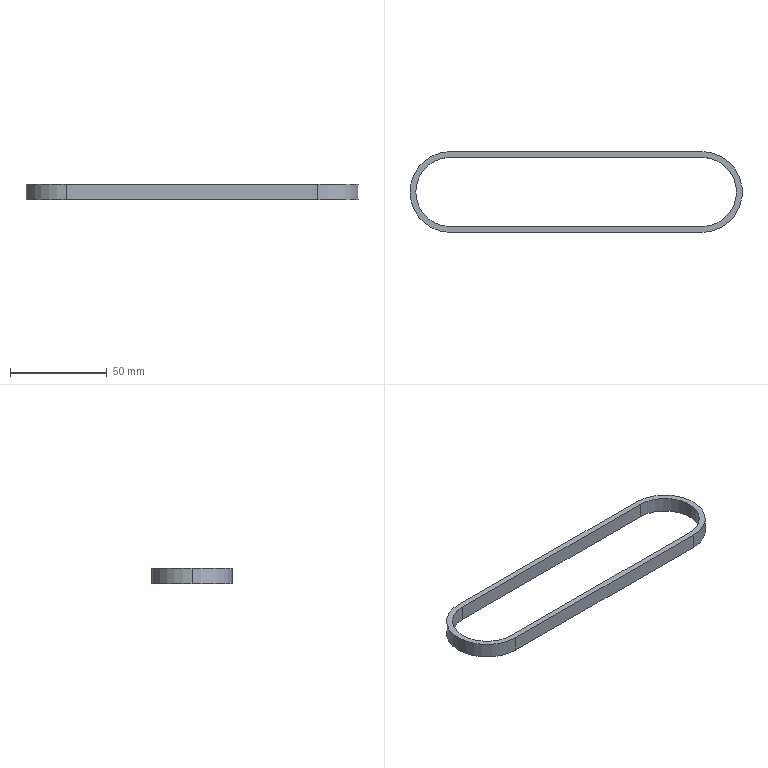Part | SolidWorks | features Extrusion 1, Shell 1 | 1 solid | 12 faces | box 171.8 x 41.8 x 7.9 mm | volume 9051 mm3 | cylinder 6 | plane 6 | commonest cylinder face diameters 35.8 x3 41.8 x3
STEP:
#1=CARTESIAN_POINT('',(-130.,17.9,7.9));
#2=VERTEX_POINT('',#1);
#3=CARTESIAN_POINT('',(-147.9,0.,7.9));
#4=VERTEX_POINT('',#3);
#5=CARTESIAN_POINT('',(-130.,0.,7.9));
#6=DIRECTION('',(0.,0.,1.));
#7=DIRECTION('',(1.,0.,0.));
#8=AXIS2_PLACEMENT_3D('',#5,#6,#7);
#9=CIRCLE('',#8,17.9);
#10=EDGE_CURVE('',#2,#4,#9,.T.);
#11=ORIENTED_EDGE('',*,*,#10,.T.);
#12=CARTESIAN_POINT('',(-147.9,0.,0.));
#13=VERTEX_POINT('',#12);
#14=CARTESIAN_POINT('',(-147.9,0.,7.9));
#15=DIRECTION('',(0.,0.,-1.));
#16=VECTOR('',#15,1000.);
#17=LINE('',#14,#16);
#18=EDGE_CURVE('',#4,#13,#17,.T.);
#19=ORIENTED_EDGE('',*,*,#18,.T.);
#20=CARTESIAN_POINT('',(-130.,17.9,0.));
#21=VERTEX_POINT('',#20);
#22=CARTESIAN_POINT('',(-130.,0.,0.));
#23=DIRECTION('',(0.,0.,1.));
#24=DIRECTION('',(1.,0.,0.));
#25=AXIS2_PLACEMENT_3D('',#22,#23,#24);
#26=CIRCLE('',#25,17.9);
#27=EDGE_CURVE('',#21,#13,#26,.T.);
#28=ORIENTED_EDGE('',*,*,#27,.F.);
#29=CARTESIAN_POINT('',(-130.,17.9,7.9));
#30=DIRECTION('',(0.,0.,-1.));
#31=VECTOR('',#30,1000.);
#32=LINE('',#29,#31);
#33=EDGE_CURVE('',#2,#21,#32,.T.);
#34=ORIENTED_EDGE('',*,*,#33,.F.);
#35=EDGE_LOOP('',(#11,#19,#28,#34));
#36=FACE_OUTER_BOUND('',#35,.T.);
#37=CARTESIAN_POINT('',(-130.,0.,7.9));
#38=DIRECTION('',(0.,0.,-1.));
#39=DIRECTION('',(-1.,0.,0.));
#40=AXIS2_PLACEMENT_3D('',#37,#38,#39);
#41=CYLINDRICAL_SURFACE('',#40,17.9);
#42=ADVANCED_FACE('',(#36),#41,.F.);
#43=CARTESIAN_POINT('',(-150.9,0.,7.9));
#44=VERTEX_POINT('',#43);
#45=CARTESIAN_POINT('',(-130.,-20.9,7.9));
#46=VERTEX_POINT('',#45);
#47=CARTESIAN_POINT('',(-130.,0.,7.9));
#48=DIRECTION('',(0.,0.,1.));
#49=DIRECTION('',(1.,0.,0.));
#50=AXIS2_PLACEMENT_3D('',#47,#48,#49);
#51=CIRCLE('',#50,20.9);
#52=EDGE_CURVE('',#44,#46,#51,.T.);
#53=ORIENTED_EDGE('',*,*,#52,.F.);
#54=CARTESIAN_POINT('',(-150.9,0.,0.));
#55=VERTEX_POINT('',#54);
#56=CARTESIAN_POINT('',(-150.9,0.,7.9));
#57=DIRECTION('',(0.,0.,-1.));
#58=VECTOR('',#57,1000.);
#59=LINE('',#56,#58);
#60=EDGE_CURVE('',#44,#55,#59,.T.);
#61=ORIENTED_EDGE('',*,*,#60,.T.);
#62=CARTESIAN_POINT('',(-130.,-20.9,0.));
#63=VERTEX_POINT('',#62);
#64=CARTESIAN_POINT('',(-130.,0.,0.));
#65=DIRECTION('',(0.,0.,1.));
#66=DIRECTION('',(1.,0.,0.));
#67=AXIS2_PLACEMENT_3D('',#64,#65,#66);
#68=CIRCLE('',#67,20.9);
#69=EDGE_CURVE('',#55,#63,#68,.T.);
#70=ORIENTED_EDGE('',*,*,#69,.T.);
#71=CARTESIAN_POINT('',(-130.,-20.9,7.9));
#72=DIRECTION('',(0.,0.,-1.));
#73=VECTOR('',#72,1000.);
#74=LINE('',#71,#73);
#75=EDGE_CURVE('',#46,#63,#74,.T.);
#76=ORIENTED_EDGE('',*,*,#75,.F.);
#77=EDGE_LOOP('',(#53,#61,#70,#76));
#78=FACE_OUTER_BOUND('',#77,.T.);
#79=CARTESIAN_POINT('',(-130.,0.,7.9));
#80=DIRECTION('',(0.,0.,-1.));
#81=DIRECTION('',(-1.,0.,0.));
#82=AXIS2_PLACEMENT_3D('',#79,#80,#81);
#83=CYLINDRICAL_SURFACE('',#82,20.9);
#84=ADVANCED_FACE('',(#78),#83,.T.);
#85=CARTESIAN_POINT('',(0.,-20.9,0.));
#86=VERTEX_POINT('',#85);
#87=CARTESIAN_POINT('',(0.,20.9,0.));
#88=VERTEX_POINT('',#87);
#89=CARTESIAN_POINT('',(0.,0.,0.));
#90=DIRECTION('',(0.,0.,1.));
#91=DIRECTION('',(1.,0.,0.));
#92=AXIS2_PLACEMENT_3D('',#89,#90,#91);
#93=CIRCLE('',#92,20.9);
#94=EDGE_CURVE('',#86,#88,#93,.T.);
#95=ORIENTED_EDGE('',*,*,#94,.T.);
#96=CARTESIAN_POINT('',(0.,20.9,7.9));
#97=VERTEX_POINT('',#96);
#98=CARTESIAN_POINT('',(0.,20.9,7.9));
#99=DIRECTION('',(0.,0.,-1.));
#100=VECTOR('',#99,1000.);
#101=LINE('',#98,#100);
#102=EDGE_CURVE('',#97,#88,#101,.T.);
#103=ORIENTED_EDGE('',*,*,#102,.F.);
#104=CARTESIAN_POINT('',(0.,-20.9,7.9));
#105=VERTEX_POINT('',#104);
#106=CARTESIAN_POINT('',(0.,0.,7.9));
#107=DIRECTION('',(0.,0.,1.));
#108=DIRECTION('',(1.,0.,0.));
#109=AXIS2_PLACEMENT_3D('',#106,#107,#108);
#110=CIRCLE('',#109,20.9);
#111=EDGE_CURVE('',#105,#97,#110,.T.);
#112=ORIENTED_EDGE('',*,*,#111,.F.);
#113=CARTESIAN_POINT('',(0.,-20.9,7.9));
#114=DIRECTION('',(0.,0.,-1.));
#115=VECTOR('',#114,1000.);
#116=LINE('',#113,#115);
#117=EDGE_CURVE('',#105,#86,#116,.T.);
#118=ORIENTED_EDGE('',*,*,#117,.T.);
#119=EDGE_LOOP('',(#95,#103,#112,#118));
#120=FACE_OUTER_BOUND('',#119,.T.);
#121=CARTESIAN_POINT('',(0.,0.,7.9));
#122=DIRECTION('',(0.,0.,-1.));
#123=DIRECTION('',(-1.,0.,0.));
#124=AXIS2_PLACEMENT_3D('',#121,#122,#123);
#125=CYLINDRICAL_SURFACE('',#124,20.9);
#126=ADVANCED_FACE('',(#120),#125,.T.);
#127=CARTESIAN_POINT('',(-130.,20.9,0.));
#128=VERTEX_POINT('',#127);
#129=CARTESIAN_POINT('',(0.,20.9,0.));
#130=DIRECTION('',(-1.,0.,0.));
#131=VECTOR('',#130,1000.);
#132=LINE('',#129,#131);
#133=EDGE_CURVE('',#88,#128,#132,.T.);
#134=ORIENTED_EDGE('',*,*,#133,.T.);
#135=CARTESIAN_POINT('',(-130.,20.9,7.9));
#136=VERTEX_POINT('',#135);
#137=CARTESIAN_POINT('',(-130.,20.9,7.9));
#138=DIRECTION('',(0.,0.,-1.));
#139=VECTOR('',#138,1000.);
#140=LINE('',#137,#139);
#141=EDGE_CURVE('',#136,#128,#140,.T.);
#142=ORIENTED_EDGE('',*,*,#141,.F.);
#143=CARTESIAN_POINT('',(0.,20.9,7.9));
#144=DIRECTION('',(-1.,0.,0.));
#145=VECTOR('',#144,1000.);
#146=LINE('',#143,#145);
#147=EDGE_CURVE('',#97,#136,#146,.T.);
#148=ORIENTED_EDGE('',*,*,#147,.F.);
#149=ORIENTED_EDGE('',*,*,#102,.T.);
#150=EDGE_LOOP('',(#134,#142,#148,#149));
#151=FACE_OUTER_BOUND('',#150,.T.);
#152=CARTESIAN_POINT('',(0.,20.9,7.9));
#153=DIRECTION('',(0.,-1.,0.));
#154=DIRECTION('',(0.,0.,-1.));
#155=AXIS2_PLACEMENT_3D('',#152,#153,#154);
#156=PLANE('',#155);
#157=ADVANCED_FACE('',(#151),#156,.F.);
#158=ORIENTED_EDGE('',*,*,#60,.F.);
#159=CARTESIAN_POINT('',(-130.,0.,7.9));
#160=DIRECTION('',(0.,0.,1.));
#161=DIRECTION('',(1.,0.,0.));
#162=AXIS2_PLACEMENT_3D('',#159,#160,#161);
#163=CIRCLE('',#162,20.9);
#164=EDGE_CURVE('',#136,#44,#163,.T.);
#165=ORIENTED_EDGE('',*,*,#164,.F.);
#166=ORIENTED_EDGE('',*,*,#141,.T.);
#167=CARTESIAN_POINT('',(-130.,0.,0.));
#168=DIRECTION('',(0.,0.,1.));
#169=DIRECTION('',(1.,0.,0.));
#170=AXIS2_PLACEMENT_3D('',#167,#168,#169);
#171=CIRCLE('',#170,20.9);
#172=EDGE_CURVE('',#128,#55,#171,.T.);
#173=ORIENTED_EDGE('',*,*,#172,.T.);
#174=EDGE_LOOP('',(#158,#165,#166,#173));
#175=FACE_OUTER_BOUND('',#174,.T.);
#176=CARTESIAN_POINT('',(-130.,0.,7.9));
#177=DIRECTION('',(0.,0.,-1.));
#178=DIRECTION('',(-1.,0.,0.));
#179=AXIS2_PLACEMENT_3D('',#176,#177,#178);
#180=CYLINDRICAL_SURFACE('',#179,20.9);
#181=ADVANCED_FACE('',(#175),#180,.T.);
#182=CARTESIAN_POINT('',(0.,-20.9,0.));
#183=DIRECTION('',(1.,0.,0.));
#184=VECTOR('',#183,1000.);
#185=LINE('',#182,#184);
#186=EDGE_CURVE('',#63,#86,#185,.T.);
#187=ORIENTED_EDGE('',*,*,#186,.T.);
#188=ORIENTED_EDGE('',*,*,#117,.F.);
#189=CARTESIAN_POINT('',(0.,-20.9,7.9));
#190=DIRECTION('',(1.,0.,0.));
#191=VECTOR('',#190,1000.);
#192=LINE('',#189,#191);
#193=EDGE_CURVE('',#46,#105,#192,.T.);
#194=ORIENTED_EDGE('',*,*,#193,.F.);
#195=ORIENTED_EDGE('',*,*,#75,.T.);
#196=EDGE_LOOP('',(#187,#188,#194,#195));
#197=FACE_OUTER_BOUND('',#196,.T.);
#198=CARTESIAN_POINT('',(0.,-20.9,7.9));
#199=DIRECTION('',(0.,1.,0.));
#200=DIRECTION('',(0.,0.,1.));
#201=AXIS2_PLACEMENT_3D('',#198,#199,#200);
#202=PLANE('',#201);
#203=ADVANCED_FACE('',(#197),#202,.F.);
#204=CARTESIAN_POINT('',(0.,-17.9,7.9));
#205=VERTEX_POINT('',#204);
#206=CARTESIAN_POINT('',(0.,17.9,7.9));
#207=VERTEX_POINT('',#206);
#208=CARTESIAN_POINT('',(0.,0.,7.9));
#209=DIRECTION('',(0.,0.,1.));
#210=DIRECTION('',(1.,0.,0.));
#211=AXIS2_PLACEMENT_3D('',#208,#209,#210);
#212=CIRCLE('',#211,17.9);
#213=EDGE_CURVE('',#205,#207,#212,.T.);
#214=ORIENTED_EDGE('',*,*,#213,.F.);
#215=CARTESIAN_POINT('',(-130.,-17.9,7.9));
#216=VERTEX_POINT('',#215);
#217=CARTESIAN_POINT('',(0.,-17.9,7.9));
#218=DIRECTION('',(1.,0.,0.));
#219=VECTOR('',#218,1000.);
#220=LINE('',#217,#219);
#221=EDGE_CURVE('',#216,#205,#220,.T.);
#222=ORIENTED_EDGE('',*,*,#221,.F.);
#223=CARTESIAN_POINT('',(-130.,0.,7.9));
#224=DIRECTION('',(0.,0.,1.));
#225=DIRECTION('',(1.,0.,0.));
#226=AXIS2_PLACEMENT_3D('',#223,#224,#225);
#227=CIRCLE('',#226,17.9);
#228=EDGE_CURVE('',#4,#216,#227,.T.);
#229=ORIENTED_EDGE('',*,*,#228,.F.);
#230=ORIENTED_EDGE('',*,*,#10,.F.);
#231=CARTESIAN_POINT('',(0.,17.9,7.9));
#232=DIRECTION('',(-1.,0.,0.));
#233=VECTOR('',#232,1000.);
#234=LINE('',#231,#233);
#235=EDGE_CURVE('',#207,#2,#234,.T.);
#236=ORIENTED_EDGE('',*,*,#235,.F.);
#237=EDGE_LOOP('',(#214,#222,#229,#230,#236));
#238=FACE_BOUND('',#237,.T.);
#239=ORIENTED_EDGE('',*,*,#111,.T.);
#240=ORIENTED_EDGE('',*,*,#147,.T.);
#241=ORIENTED_EDGE('',*,*,#164,.T.);
#242=ORIENTED_EDGE('',*,*,#52,.T.);
#243=ORIENTED_EDGE('',*,*,#193,.T.);
#244=EDGE_LOOP('',(#239,#240,#241,#242,#243));
#245=FACE_OUTER_BOUND('',#244,.T.);
#246=CARTESIAN_POINT('',(0.,0.,7.9));
#247=DIRECTION('',(0.,0.,1.));
#248=DIRECTION('',(1.,0.,0.));
#249=AXIS2_PLACEMENT_3D('',#246,#247,#248);
#250=PLANE('',#249);
#251=ADVANCED_FACE('',(#238,#245),#250,.T.);
#252=CARTESIAN_POINT('',(-130.,-17.9,0.));
#253=VERTEX_POINT('',#252);
#254=CARTESIAN_POINT('',(0.,-17.9,0.));
#255=VERTEX_POINT('',#254);
#256=CARTESIAN_POINT('',(0.,-17.9,0.));
#257=DIRECTION('',(1.,0.,0.));
#258=VECTOR('',#257,1000.);
#259=LINE('',#256,#258);
#260=EDGE_CURVE('',#253,#255,#259,.T.);
#261=ORIENTED_EDGE('',*,*,#260,.T.);
#262=CARTESIAN_POINT('',(0.,17.9,0.));
#263=VERTEX_POINT('',#262);
#264=CARTESIAN_POINT('',(0.,0.,0.));
#265=DIRECTION('',(0.,0.,1.));
#266=DIRECTION('',(1.,0.,0.));
#267=AXIS2_PLACEMENT_3D('',#264,#265,#266);
#268=CIRCLE('',#267,17.9);
#269=EDGE_CURVE('',#255,#263,#268,.T.);
#270=ORIENTED_EDGE('',*,*,#269,.T.);
#271=CARTESIAN_POINT('',(0.,17.9,0.));
#272=DIRECTION('',(-1.,0.,0.));
#273=VECTOR('',#272,1000.);
#274=LINE('',#271,#273);
#275=EDGE_CURVE('',#263,#21,#274,.T.);
#276=ORIENTED_EDGE('',*,*,#275,.T.);
#277=ORIENTED_EDGE('',*,*,#27,.T.);
#278=CARTESIAN_POINT('',(-130.,0.,0.));
#279=DIRECTION('',(0.,0.,1.));
#280=DIRECTION('',(1.,0.,0.));
#281=AXIS2_PLACEMENT_3D('',#278,#279,#280);
#282=CIRCLE('',#281,17.9);
#283=EDGE_CURVE('',#13,#253,#282,.T.);
#284=ORIENTED_EDGE('',*,*,#283,.T.);
#285=EDGE_LOOP('',(#261,#270,#276,#277,#284));
#286=FACE_BOUND('',#285,.T.);
#287=ORIENTED_EDGE('',*,*,#94,.F.);
#288=ORIENTED_EDGE('',*,*,#186,.F.);
#289=ORIENTED_EDGE('',*,*,#69,.F.);
#290=ORIENTED_EDGE('',*,*,#172,.F.);
#291=ORIENTED_EDGE('',*,*,#133,.F.);
#292=EDGE_LOOP('',(#287,#288,#289,#290,#291));
#293=FACE_OUTER_BOUND('',#292,.T.);
#294=CARTESIAN_POINT('',(0.,0.,0.));
#295=DIRECTION('',(0.,0.,1.));
#296=DIRECTION('',(1.,0.,0.));
#297=AXIS2_PLACEMENT_3D('',#294,#295,#296);
#298=PLANE('',#297);
#299=ADVANCED_FACE('',(#286,#293),#298,.F.);
#300=ORIENTED_EDGE('',*,*,#269,.F.);
#301=CARTESIAN_POINT('',(0.,-17.9,7.9));
#302=DIRECTION('',(0.,0.,-1.));
#303=VECTOR('',#302,1000.);
#304=LINE('',#301,#303);
#305=EDGE_CURVE('',#205,#255,#304,.T.);
#306=ORIENTED_EDGE('',*,*,#305,.F.);
#307=ORIENTED_EDGE('',*,*,#213,.T.);
#308=CARTESIAN_POINT('',(0.,17.9,7.9));
#309=DIRECTION('',(0.,0.,-1.));
#310=VECTOR('',#309,1000.);
#311=LINE('',#308,#310);
#312=EDGE_CURVE('',#207,#263,#311,.T.);
#313=ORIENTED_EDGE('',*,*,#312,.T.);
#314=EDGE_LOOP('',(#300,#306,#307,#313));
#315=FACE_OUTER_BOUND('',#314,.T.);
#316=CARTESIAN_POINT('',(0.,0.,7.9));
#317=DIRECTION('',(0.,0.,-1.));
#318=DIRECTION('',(-1.,0.,0.));
#319=AXIS2_PLACEMENT_3D('',#316,#317,#318);
#320=CYLINDRICAL_SURFACE('',#319,17.9);
#321=ADVANCED_FACE('',(#315),#320,.F.);
#322=ORIENTED_EDGE('',*,*,#275,.F.);
#323=ORIENTED_EDGE('',*,*,#312,.F.);
#324=ORIENTED_EDGE('',*,*,#235,.T.);
#325=ORIENTED_EDGE('',*,*,#33,.T.);
#326=EDGE_LOOP('',(#322,#323,#324,#325));
#327=FACE_OUTER_BOUND('',#326,.T.);
#328=CARTESIAN_POINT('',(0.,17.9,7.9));
#329=DIRECTION('',(0.,-1.,0.));
#330=DIRECTION('',(0.,0.,-1.));
#331=AXIS2_PLACEMENT_3D('',#328,#329,#330);
#332=PLANE('',#331);
#333=ADVANCED_FACE('',(#327),#332,.T.);
#334=ORIENTED_EDGE('',*,*,#18,.F.);
#335=ORIENTED_EDGE('',*,*,#228,.T.);
#336=CARTESIAN_POINT('',(-130.,-17.9,7.9));
#337=DIRECTION('',(0.,0.,-1.));
#338=VECTOR('',#337,1000.);
#339=LINE('',#336,#338);
#340=EDGE_CURVE('',#216,#253,#339,.T.);
#341=ORIENTED_EDGE('',*,*,#340,.T.);
#342=ORIENTED_EDGE('',*,*,#283,.F.);
#343=EDGE_LOOP('',(#334,#335,#341,#342));
#344=FACE_OUTER_BOUND('',#343,.T.);
#345=CARTESIAN_POINT('',(-130.,0.,7.9));
#346=DIRECTION('',(0.,0.,-1.));
#347=DIRECTION('',(-1.,0.,0.));
#348=AXIS2_PLACEMENT_3D('',#345,#346,#347);
#349=CYLINDRICAL_SURFACE('',#348,17.9);
#350=ADVANCED_FACE('',(#344),#349,.F.);
#351=ORIENTED_EDGE('',*,*,#260,.F.);
#352=ORIENTED_EDGE('',*,*,#340,.F.);
#353=ORIENTED_EDGE('',*,*,#221,.T.);
#354=ORIENTED_EDGE('',*,*,#305,.T.);
#355=EDGE_LOOP('',(#351,#352,#353,#354));
#356=FACE_OUTER_BOUND('',#355,.T.);
#357=CARTESIAN_POINT('',(0.,-17.9,7.9));
#358=DIRECTION('',(0.,1.,0.));
#359=DIRECTION('',(0.,0.,1.));
#360=AXIS2_PLACEMENT_3D('',#357,#358,#359);
#361=PLANE('',#360);
#362=ADVANCED_FACE('',(#356),#361,.T.);
#363=CLOSED_SHELL('',(#42,#84,#126,#157,#181,#203,#251,#299,#321,#333,#350,#362));
#364=MANIFOLD_SOLID_BREP('',#363);
#365=CARTESIAN_POINT('',(0.,0.,0.));
#366=DIRECTION('',(0.,0.,1.));
#367=DIRECTION('',(1.,0.,0.));
#368=AXIS2_PLACEMENT_3D('',#365,#366,#367);
#369=(LENGTH_UNIT()NAMED_UNIT(*)SI_UNIT(.MILLI.,.METRE.));
#370=UNCERTAINTY_MEASURE_WITH_UNIT(LENGTH_MEASURE(0.00001),#369,'','');
#371=(NAMED_UNIT(*)PLANE_ANGLE_UNIT()SI_UNIT($,.RADIAN.));
#372=(NAMED_UNIT(*)SI_UNIT($,.STERADIAN.)SOLID_ANGLE_UNIT());
#373=(GEOMETRIC_REPRESENTATION_CONTEXT(3)GLOBAL_UNCERTAINTY_ASSIGNED_CONTEXT((#370))GLOBAL_UNIT_ASSIGNED_CONTEXT((#369,#371,#372))REPRESENTATION_CONTEXT('',''));
#374=ADVANCED_BREP_SHAPE_REPRESENTATION('',(#364,#368),#373);